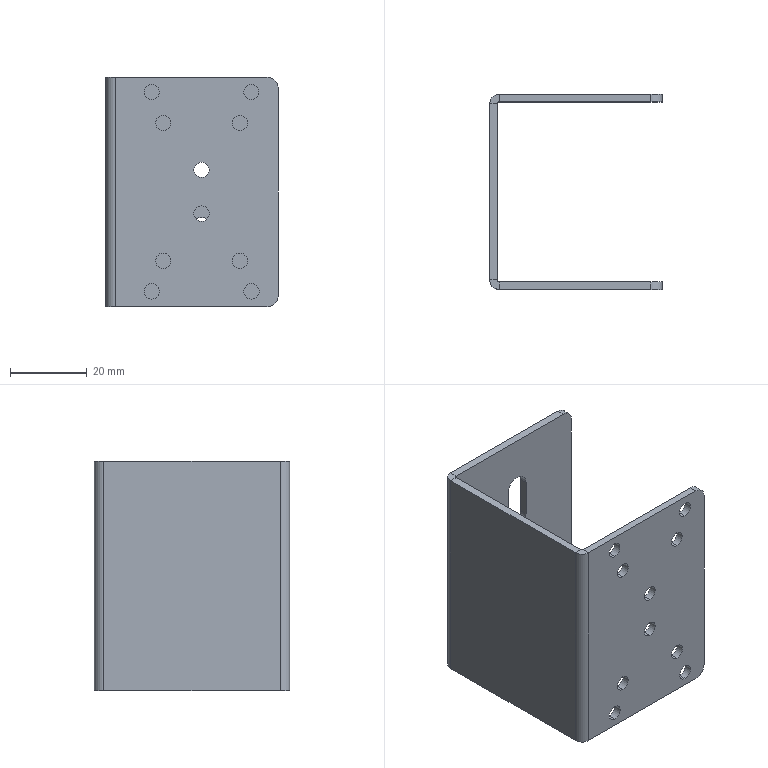Part | SolidWorks | features ICE 2, ExtruThin 1, Fillet 1, FlatPattern 1, FlattenBends 1, ProcessBends 1, SheetMetal 1 | 1 solid | 56 faces | box 45 x 51 x 60 mm | volume 15618 mm3 | cylinder 34 | plane 22 | commonest cylinder face diameters 4 x20 6.6 x6 6 x4 1 x2 5 x2